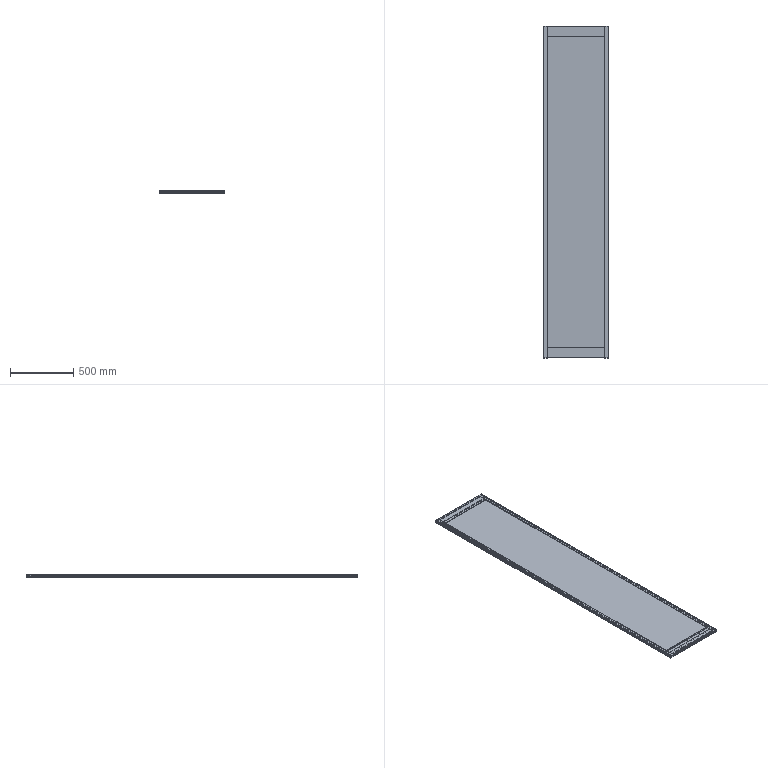Part | 5 solids | 365 faces | box 510 x 2616 x 20.2 mm | volume 13127728 mm3 | cylinder 191 | plane 174 | commonest cylinder face diameters 0.6 x48 13 x48 0.4 x34 1 x21 9 x16 7.2 x12